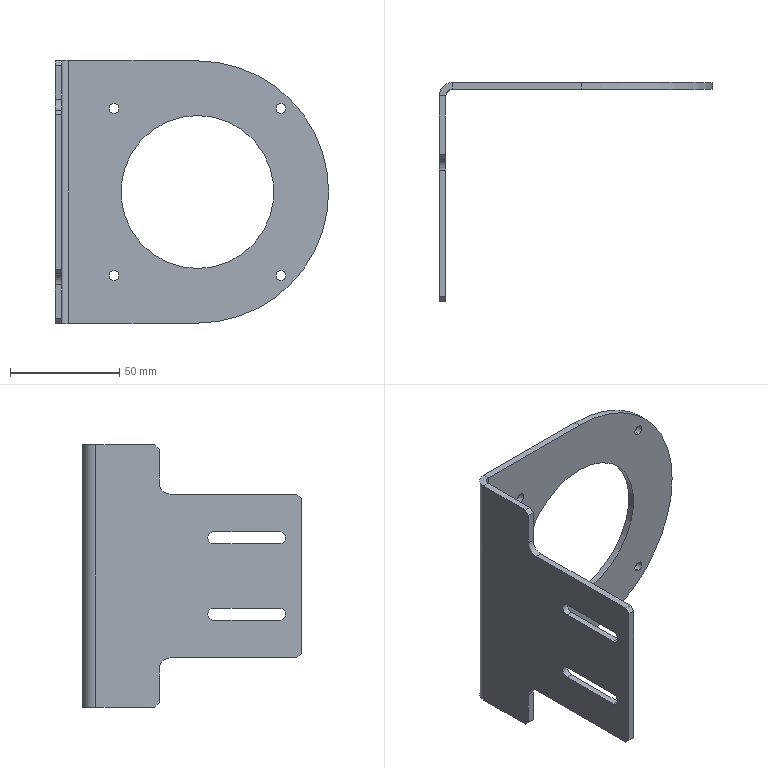Part | SolidWorks | features ICE 3, HoleWzd 2, Chamfer 1, EdgeFlange 1, Fillet 1, FlatPattern 1, MirrorSolid 1, SMBaseFlange 1, SheetMetal 1 | 1 solid | 42 faces | box 125 x 100 x 120 mm | volume 52954 mm3 | plane 23 | cylinder 19 | commonest cylinder face diameters 4.5 x8 5.5 x4 10 x2 70 x2 6 x1 12 x1
STEP:
#1=CARTESIAN_POINT('',(38.184,-3.,-40.434));
#2=VERTEX_POINT('',#1);
#3=CARTESIAN_POINT('',(38.184,-3.,-35.934));
#4=VERTEX_POINT('',#3);
#5=CARTESIAN_POINT('',(38.184,-3.,-38.184));
#6=DIRECTION('',(0.,1.,0.));
#7=DIRECTION('',(0.,0.,1.));
#8=AXIS2_PLACEMENT_3D('',#5,#6,#7);
#9=CIRCLE('',#8,2.25);
#10=EDGE_CURVE('',#2,#4,#9,.T.);
#11=ORIENTED_EDGE('',*,*,#10,.F.);
#12=CARTESIAN_POINT('',(38.184,0.,-40.434));
#13=VERTEX_POINT('',#12);
#14=CARTESIAN_POINT('',(38.184,0.,-40.434));
#15=DIRECTION('',(0.,1.,0.));
#16=VECTOR('',#15,1000.);
#17=LINE('',#14,#16);
#18=EDGE_CURVE('',#2,#13,#17,.T.);
#19=ORIENTED_EDGE('',*,*,#18,.T.);
#20=CARTESIAN_POINT('',(38.184,0.,-35.934));
#21=VERTEX_POINT('',#20);
#22=CARTESIAN_POINT('',(38.184,0.,-38.184));
#23=DIRECTION('',(0.,1.,0.));
#24=DIRECTION('',(0.,0.,1.));
#25=AXIS2_PLACEMENT_3D('',#22,#23,#24);
#26=CIRCLE('',#25,2.25);
#27=EDGE_CURVE('',#13,#21,#26,.T.);
#28=ORIENTED_EDGE('',*,*,#27,.T.);
#29=CARTESIAN_POINT('',(38.184,0.,-35.934));
#30=DIRECTION('',(0.,1.,0.));
#31=VECTOR('',#30,1000.);
#32=LINE('',#29,#31);
#33=EDGE_CURVE('',#4,#21,#32,.T.);
#34=ORIENTED_EDGE('',*,*,#33,.F.);
#35=EDGE_LOOP('',(#11,#19,#28,#34));
#36=FACE_OUTER_BOUND('',#35,.T.);
#37=CARTESIAN_POINT('',(38.184,0.,-38.184));
#38=DIRECTION('',(0.,1.,0.));
#39=DIRECTION('',(0.,0.,1.));
#40=AXIS2_PLACEMENT_3D('',#37,#38,#39);
#41=CYLINDRICAL_SURFACE('',#40,2.25);
#42=ADVANCED_FACE('',(#36),#41,.F.);
#43=CARTESIAN_POINT('',(38.184,-3.,35.934));
#44=VERTEX_POINT('',#43);
#45=CARTESIAN_POINT('',(38.184,-3.,40.434));
#46=VERTEX_POINT('',#45);
#47=CARTESIAN_POINT('',(38.184,-3.,38.184));
#48=DIRECTION('',(0.,1.,0.));
#49=DIRECTION('',(0.,0.,1.));
#50=AXIS2_PLACEMENT_3D('',#47,#48,#49);
#51=CIRCLE('',#50,2.25);
#52=EDGE_CURVE('',#44,#46,#51,.T.);
#53=ORIENTED_EDGE('',*,*,#52,.F.);
#54=CARTESIAN_POINT('',(38.184,0.,35.934));
#55=VERTEX_POINT('',#54);
#56=CARTESIAN_POINT('',(38.184,0.,35.934));
#57=DIRECTION('',(0.,1.,0.));
#58=VECTOR('',#57,1000.);
#59=LINE('',#56,#58);
#60=EDGE_CURVE('',#44,#55,#59,.T.);
#61=ORIENTED_EDGE('',*,*,#60,.T.);
#62=CARTESIAN_POINT('',(38.184,0.,40.434));
#63=VERTEX_POINT('',#62);
#64=CARTESIAN_POINT('',(38.184,0.,38.184));
#65=DIRECTION('',(0.,1.,0.));
#66=DIRECTION('',(0.,0.,1.));
#67=AXIS2_PLACEMENT_3D('',#64,#65,#66);
#68=CIRCLE('',#67,2.25);
#69=EDGE_CURVE('',#55,#63,#68,.T.);
#70=ORIENTED_EDGE('',*,*,#69,.T.);
#71=CARTESIAN_POINT('',(38.184,0.,40.434));
#72=DIRECTION('',(0.,1.,0.));
#73=VECTOR('',#72,1000.);
#74=LINE('',#71,#73);
#75=EDGE_CURVE('',#46,#63,#74,.T.);
#76=ORIENTED_EDGE('',*,*,#75,.F.);
#77=EDGE_LOOP('',(#53,#61,#70,#76));
#78=FACE_OUTER_BOUND('',#77,.T.);
#79=CARTESIAN_POINT('',(38.184,0.,38.184));
#80=DIRECTION('',(0.,1.,0.));
#81=DIRECTION('',(0.,0.,1.));
#82=AXIS2_PLACEMENT_3D('',#79,#80,#81);
#83=CYLINDRICAL_SURFACE('',#82,2.25);
#84=ADVANCED_FACE('',(#78),#83,.F.);
#85=CARTESIAN_POINT('',(-38.184,-3.,35.934));
#86=VERTEX_POINT('',#85);
#87=CARTESIAN_POINT('',(-38.184,-3.,40.434));
#88=VERTEX_POINT('',#87);
#89=CARTESIAN_POINT('',(-38.184,-3.,38.184));
#90=DIRECTION('',(0.,1.,0.));
#91=DIRECTION('',(0.,0.,1.));
#92=AXIS2_PLACEMENT_3D('',#89,#90,#91);
#93=CIRCLE('',#92,2.25);
#94=EDGE_CURVE('',#86,#88,#93,.T.);
#95=ORIENTED_EDGE('',*,*,#94,.F.);
#96=CARTESIAN_POINT('',(-38.184,0.,35.934));
#97=VERTEX_POINT('',#96);
#98=CARTESIAN_POINT('',(-38.184,0.,35.934));
#99=DIRECTION('',(0.,1.,0.));
#100=VECTOR('',#99,1000.);
#101=LINE('',#98,#100);
#102=EDGE_CURVE('',#86,#97,#101,.T.);
#103=ORIENTED_EDGE('',*,*,#102,.T.);
#104=CARTESIAN_POINT('',(-38.184,0.,40.434));
#105=VERTEX_POINT('',#104);
#106=CARTESIAN_POINT('',(-38.184,0.,38.184));
#107=DIRECTION('',(0.,1.,0.));
#108=DIRECTION('',(0.,0.,1.));
#109=AXIS2_PLACEMENT_3D('',#106,#107,#108);
#110=CIRCLE('',#109,2.25);
#111=EDGE_CURVE('',#97,#105,#110,.T.);
#112=ORIENTED_EDGE('',*,*,#111,.T.);
#113=CARTESIAN_POINT('',(-38.184,0.,40.434));
#114=DIRECTION('',(0.,1.,0.));
#115=VECTOR('',#114,1000.);
#116=LINE('',#113,#115);
#117=EDGE_CURVE('',#88,#105,#116,.T.);
#118=ORIENTED_EDGE('',*,*,#117,.F.);
#119=EDGE_LOOP('',(#95,#103,#112,#118));
#120=FACE_OUTER_BOUND('',#119,.T.);
#121=CARTESIAN_POINT('',(-38.184,0.,38.184));
#122=DIRECTION('',(0.,1.,0.));
#123=DIRECTION('',(0.,0.,1.));
#124=AXIS2_PLACEMENT_3D('',#121,#122,#123);
#125=CYLINDRICAL_SURFACE('',#124,2.25);
#126=ADVANCED_FACE('',(#120),#125,.F.);
#127=CARTESIAN_POINT('',(-38.184,-3.,-40.434));
#128=VERTEX_POINT('',#127);
#129=CARTESIAN_POINT('',(-38.184,-3.,-35.934));
#130=VERTEX_POINT('',#129);
#131=CARTESIAN_POINT('',(-38.184,-3.,-38.184));
#132=DIRECTION('',(0.,1.,0.));
#133=DIRECTION('',(0.,0.,1.));
#134=AXIS2_PLACEMENT_3D('',#131,#132,#133);
#135=CIRCLE('',#134,2.25);
#136=EDGE_CURVE('',#128,#130,#135,.T.);
#137=ORIENTED_EDGE('',*,*,#136,.F.);
#138=CARTESIAN_POINT('',(-38.184,0.,-40.434));
#139=VERTEX_POINT('',#138);
#140=CARTESIAN_POINT('',(-38.184,0.,-40.434));
#141=DIRECTION('',(0.,1.,0.));
#142=VECTOR('',#141,1000.);
#143=LINE('',#140,#142);
#144=EDGE_CURVE('',#128,#139,#143,.T.);
#145=ORIENTED_EDGE('',*,*,#144,.T.);
#146=CARTESIAN_POINT('',(-38.184,0.,-35.934));
#147=VERTEX_POINT('',#146);
#148=CARTESIAN_POINT('',(-38.184,0.,-38.184));
#149=DIRECTION('',(0.,1.,0.));
#150=DIRECTION('',(0.,0.,1.));
#151=AXIS2_PLACEMENT_3D('',#148,#149,#150);
#152=CIRCLE('',#151,2.25);
#153=EDGE_CURVE('',#139,#147,#152,.T.);
#154=ORIENTED_EDGE('',*,*,#153,.T.);
#155=CARTESIAN_POINT('',(-38.184,0.,-35.934));
#156=DIRECTION('',(0.,1.,0.));
#157=VECTOR('',#156,1000.);
#158=LINE('',#155,#157);
#159=EDGE_CURVE('',#130,#147,#158,.T.);
#160=ORIENTED_EDGE('',*,*,#159,.F.);
#161=EDGE_LOOP('',(#137,#145,#154,#160));
#162=FACE_OUTER_BOUND('',#161,.T.);
#163=CARTESIAN_POINT('',(-38.184,0.,-38.184));
#164=DIRECTION('',(0.,1.,0.));
#165=DIRECTION('',(0.,0.,1.));
#166=AXIS2_PLACEMENT_3D('',#163,#164,#165);
#167=CYLINDRICAL_SURFACE('',#166,2.25);
#168=ADVANCED_FACE('',(#162),#167,.F.);
#169=CARTESIAN_POINT('',(0.,-3.,-35.));
#170=VERTEX_POINT('',#169);
#171=CARTESIAN_POINT('',(0.,-3.,35.));
#172=VERTEX_POINT('',#171);
#173=CARTESIAN_POINT('',(0.,-3.,0.));
#174=DIRECTION('',(0.,1.,0.));
#175=DIRECTION('',(0.,0.,1.));
#176=AXIS2_PLACEMENT_3D('',#173,#174,#175);
#177=CIRCLE('',#176,35.);
#178=EDGE_CURVE('',#170,#172,#177,.T.);
#179=ORIENTED_EDGE('',*,*,#178,.F.);
#180=CARTESIAN_POINT('',(0.,0.,-35.));
#181=VERTEX_POINT('',#180);
#182=CARTESIAN_POINT('',(0.,-3.,-35.));
#183=DIRECTION('',(0.,1.,0.));
#184=VECTOR('',#183,1000.);
#185=LINE('',#182,#184);
#186=EDGE_CURVE('',#170,#181,#185,.T.);
#187=ORIENTED_EDGE('',*,*,#186,.T.);
#188=CARTESIAN_POINT('',(0.,0.,35.));
#189=VERTEX_POINT('',#188);
#190=CARTESIAN_POINT('',(0.,0.,0.));
#191=DIRECTION('',(0.,1.,0.));
#192=DIRECTION('',(0.,0.,1.));
#193=AXIS2_PLACEMENT_3D('',#190,#191,#192);
#194=CIRCLE('',#193,35.);
#195=EDGE_CURVE('',#181,#189,#194,.T.);
#196=ORIENTED_EDGE('',*,*,#195,.T.);
#197=CARTESIAN_POINT('',(0.,-3.,35.));
#198=DIRECTION('',(0.,1.,0.));
#199=VECTOR('',#198,1000.);
#200=LINE('',#197,#199);
#201=EDGE_CURVE('',#172,#189,#200,.T.);
#202=ORIENTED_EDGE('',*,*,#201,.F.);
#203=EDGE_LOOP('',(#179,#187,#196,#202));
#204=FACE_OUTER_BOUND('',#203,.T.);
#205=CARTESIAN_POINT('',(0.,-3.,0.));
#206=DIRECTION('',(0.,1.,0.));
#207=DIRECTION('',(0.,0.,1.));
#208=AXIS2_PLACEMENT_3D('',#205,#206,#207);
#209=CYLINDRICAL_SURFACE('',#208,35.);
#210=ADVANCED_FACE('',(#204),#209,.F.);
#211=CARTESIAN_POINT('',(0.,-3.,-60.));
#212=VERTEX_POINT('',#211);
#213=CARTESIAN_POINT('',(-59.,-3.,-60.));
#214=VERTEX_POINT('',#213);
#215=CARTESIAN_POINT('',(0.,-3.,-60.));
#216=DIRECTION('',(-1.,0.,0.));
#217=VECTOR('',#216,1000.);
#218=LINE('',#215,#217);
#219=EDGE_CURVE('',#212,#214,#218,.T.);
#220=ORIENTED_EDGE('',*,*,#219,.T.);
#221=CARTESIAN_POINT('',(-59.,0.,-60.));
#222=VERTEX_POINT('',#221);
#223=CARTESIAN_POINT('',(-59.,-3.,-60.));
#224=DIRECTION('',(0.,1.,0.));
#225=VECTOR('',#224,1000.);
#226=LINE('',#223,#225);
#227=EDGE_CURVE('',#214,#222,#226,.T.);
#228=ORIENTED_EDGE('',*,*,#227,.T.);
#229=CARTESIAN_POINT('',(0.,0.,-60.));
#230=VERTEX_POINT('',#229);
#231=CARTESIAN_POINT('',(0.,0.,-60.));
#232=DIRECTION('',(-1.,0.,0.));
#233=VECTOR('',#232,1000.);
#234=LINE('',#231,#233);
#235=EDGE_CURVE('',#230,#222,#234,.T.);
#236=ORIENTED_EDGE('',*,*,#235,.F.);
#237=CARTESIAN_POINT('',(0.,-3.,-60.));
#238=DIRECTION('',(0.,1.,0.));
#239=VECTOR('',#238,1000.);
#240=LINE('',#237,#239);
#241=EDGE_CURVE('',#212,#230,#240,.T.);
#242=ORIENTED_EDGE('',*,*,#241,.F.);
#243=EDGE_LOOP('',(#220,#228,#236,#242));
#244=FACE_OUTER_BOUND('',#243,.T.);
#245=CARTESIAN_POINT('',(0.,-3.,-60.));
#246=DIRECTION('',(0.,0.,-1.));
#247=DIRECTION('',(-1.,0.,0.));
#248=AXIS2_PLACEMENT_3D('',#245,#246,#247);
#249=PLANE('',#248);
#250=ADVANCED_FACE('',(#244),#249,.T.);
#251=CARTESIAN_POINT('',(38.184,-3.,-38.184));
#252=DIRECTION('',(0.,1.,0.));
#253=DIRECTION('',(0.,0.,1.));
#254=AXIS2_PLACEMENT_3D('',#251,#252,#253);
#255=CIRCLE('',#254,2.25);
#256=EDGE_CURVE('',#4,#2,#255,.T.);
#257=ORIENTED_EDGE('',*,*,#256,.T.);
#258=ORIENTED_EDGE('',*,*,#10,.T.);
#259=EDGE_LOOP('',(#257,#258));
#260=FACE_BOUND('',#259,.T.);
#261=CARTESIAN_POINT('',(38.184,-3.,38.184));
#262=DIRECTION('',(0.,1.,0.));
#263=DIRECTION('',(0.,0.,1.));
#264=AXIS2_PLACEMENT_3D('',#261,#262,#263);
#265=CIRCLE('',#264,2.25);
#266=EDGE_CURVE('',#46,#44,#265,.T.);
#267=ORIENTED_EDGE('',*,*,#266,.T.);
#268=ORIENTED_EDGE('',*,*,#52,.T.);
#269=EDGE_LOOP('',(#267,#268));
#270=FACE_BOUND('',#269,.T.);
#271=CARTESIAN_POINT('',(-38.184,-3.,38.184));
#272=DIRECTION('',(0.,1.,0.));
#273=DIRECTION('',(0.,0.,1.));
#274=AXIS2_PLACEMENT_3D('',#271,#272,#273);
#275=CIRCLE('',#274,2.25);
#276=EDGE_CURVE('',#88,#86,#275,.T.);
#277=ORIENTED_EDGE('',*,*,#276,.T.);
#278=ORIENTED_EDGE('',*,*,#94,.T.);
#279=EDGE_LOOP('',(#277,#278));
#280=FACE_BOUND('',#279,.T.);
#281=CARTESIAN_POINT('',(-38.184,-3.,-38.184));
#282=DIRECTION('',(0.,1.,0.));
#283=DIRECTION('',(0.,0.,1.));
#284=AXIS2_PLACEMENT_3D('',#281,#282,#283);
#285=CIRCLE('',#284,2.25);
#286=EDGE_CURVE('',#130,#128,#285,.T.);
#287=ORIENTED_EDGE('',*,*,#286,.T.);
#288=ORIENTED_EDGE('',*,*,#136,.T.);
#289=EDGE_LOOP('',(#287,#288));
#290=FACE_BOUND('',#289,.T.);
#291=CARTESIAN_POINT('',(0.,-3.,0.));
#292=DIRECTION('',(0.,1.,0.));
#293=DIRECTION('',(0.,0.,1.));
#294=AXIS2_PLACEMENT_3D('',#291,#292,#293);
#295=CIRCLE('',#294,35.);
#296=EDGE_CURVE('',#172,#170,#295,.T.);
#297=ORIENTED_EDGE('',*,*,#296,.T.);
#298=ORIENTED_EDGE('',*,*,#178,.T.);
#299=EDGE_LOOP('',(#297,#298));
#300=FACE_BOUND('',#299,.T.);
#301=CARTESIAN_POINT('',(-59.,-3.,60.));
#302=VERTEX_POINT('',#301);
#303=CARTESIAN_POINT('',(-59.,-3.,-60.));
#304=DIRECTION('',(0.,0.,1.));
#305=VECTOR('',#304,1000.);
#306=LINE('',#303,#305);
#307=EDGE_CURVE('',#214,#302,#306,.T.);
#308=ORIENTED_EDGE('',*,*,#307,.F.);
#309=ORIENTED_EDGE('',*,*,#219,.F.);
#310=CARTESIAN_POINT('',(0.,-3.,60.));
#311=VERTEX_POINT('',#310);
#312=CARTESIAN_POINT('',(0.,-3.,0.));
#313=DIRECTION('',(0.,1.,0.));
#314=DIRECTION('',(0.,0.,1.));
#315=AXIS2_PLACEMENT_3D('',#312,#313,#314);
#316=CIRCLE('',#315,60.);
#317=EDGE_CURVE('',#311,#212,#316,.T.);
#318=ORIENTED_EDGE('',*,*,#317,.F.);
#319=CARTESIAN_POINT('',(-65.,-3.,60.));
#320=DIRECTION('',(1.,0.,0.));
#321=VECTOR('',#320,1000.);
#322=LINE('',#319,#321);
#323=EDGE_CURVE('',#302,#311,#322,.T.);
#324=ORIENTED_EDGE('',*,*,#323,.F.);
#325=EDGE_LOOP('',(#308,#309,#318,#324));
#326=FACE_OUTER_BOUND('',#325,.T.);
#327=CARTESIAN_POINT('',(0.,-3.,0.));
#328=DIRECTION('',(0.,1.,0.));
#329=DIRECTION('',(0.,0.,1.));
#330=AXIS2_PLACEMENT_3D('',#327,#328,#329);
#331=PLANE('',#330);
#332=ADVANCED_FACE('',(#260,#270,#280,#290,#300,#326),#331,.F.);
#333=CARTESIAN_POINT('',(38.184,0.,-38.184));
#334=DIRECTION('',(0.,1.,0.));
#335=DIRECTION('',(0.,0.,1.));
#336=AXIS2_PLACEMENT_3D('',#333,#334,#335);
#337=CIRCLE('',#336,2.25);
#338=EDGE_CURVE('',#21,#13,#337,.T.);
#339=ORIENTED_EDGE('',*,*,#338,.F.);
#340=ORIENTED_EDGE('',*,*,#27,.F.);
#341=EDGE_LOOP('',(#339,#340));
#342=FACE_BOUND('',#341,.T.);
#343=CARTESIAN_POINT('',(38.184,0.,38.184));
#344=DIRECTION('',(0.,1.,0.));
#345=DIRECTION('',(0.,0.,1.));
#346=AXIS2_PLACEMENT_3D('',#343,#344,#345);
#347=CIRCLE('',#346,2.25);
#348=EDGE_CURVE('',#63,#55,#347,.T.);
#349=ORIENTED_EDGE('',*,*,#348,.F.);
#350=ORIENTED_EDGE('',*,*,#69,.F.);
#351=EDGE_LOOP('',(#349,#350));
#352=FACE_BOUND('',#351,.T.);
#353=CARTESIAN_POINT('',(-38.184,0.,38.184));
#354=DIRECTION('',(0.,1.,0.));
#355=DIRECTION('',(0.,0.,1.));
#356=AXIS2_PLACEMENT_3D('',#353,#354,#355);
#357=CIRCLE('',#356,2.25);
#358=EDGE_CURVE('',#105,#97,#357,.T.);
#359=ORIENTED_EDGE('',*,*,#358,.F.);
#360=ORIENTED_EDGE('',*,*,#111,.F.);
#361=EDGE_LOOP('',(#359,#360));
#362=FACE_BOUND('',#361,.T.);
#363=CARTESIAN_POINT('',(-38.184,0.,-38.184));
#364=DIRECTION('',(0.,1.,0.));
#365=DIRECTION('',(0.,0.,1.));
#366=AXIS2_PLACEMENT_3D('',#363,#364,#365);
#367=CIRCLE('',#366,2.25);
#368=EDGE_CURVE('',#147,#139,#367,.T.);
#369=ORIENTED_EDGE('',*,*,#368,.F.);
#370=ORIENTED_EDGE('',*,*,#153,.F.);
#371=EDGE_LOOP('',(#369,#370));
#372=FACE_BOUND('',#371,.T.);
#373=CARTESIAN_POINT('',(0.,0.,0.));
#374=DIRECTION('',(0.,1.,0.));
#375=DIRECTION('',(0.,0.,1.));
#376=AXIS2_PLACEMENT_3D('',#373,#374,#375);
#377=CIRCLE('',#376,35.);
#378=EDGE_CURVE('',#189,#181,#377,.T.);
#379=ORIENTED_EDGE('',*,*,#378,.F.);
#380=ORIENTED_EDGE('',*,*,#195,.F.);
#381=EDGE_LOOP('',(#379,#380));
#382=FACE_BOUND('',#381,.T.);
#383=ORIENTED_EDGE('',*,*,#235,.T.);
#384=CARTESIAN_POINT('',(-59.,0.,60.));
#385=VERTEX_POINT('',#384);
#386=CARTESIAN_POINT('',(-59.,0.,-60.));
#387=DIRECTION('',(0.,0.,1.));
#388=VECTOR('',#387,1000.);
#389=LINE('',#386,#388);
#390=EDGE_CURVE('',#222,#385,#389,.T.);
#391=ORIENTED_EDGE('',*,*,#390,.T.);
#392=CARTESIAN_POINT('',(0.,0.,60.));
#393=VERTEX_POINT('',#392);
#394=CARTESIAN_POINT('',(-65.,0.,60.));
#395=DIRECTION('',(1.,0.,0.));
#396=VECTOR('',#395,1000.);
#397=LINE('',#394,#396);
#398=EDGE_CURVE('',#385,#393,#397,.T.);
#399=ORIENTED_EDGE('',*,*,#398,.T.);
#400=CARTESIAN_POINT('',(0.,0.,0.));
#401=DIRECTION('',(0.,1.,0.));
#402=DIRECTION('',(0.,0.,1.));
#403=AXIS2_PLACEMENT_3D('',#400,#401,#402);
#404=CIRCLE('',#403,60.);
#405=EDGE_CURVE('',#393,#230,#404,.T.);
#406=ORIENTED_EDGE('',*,*,#405,.T.);
#407=EDGE_LOOP('',(#383,#391,#399,#406));
#408=FACE_OUTER_BOUND('',#407,.T.);
#409=CARTESIAN_POINT('',(0.,0.,0.));
#410=DIRECTION('',(0.,1.,0.));
#411=DIRECTION('',(0.,0.,1.));
#412=AXIS2_PLACEMENT_3D('',#409,#410,#411);
#413=PLANE('',#412);
#414=ADVANCED_FACE('',(#342,#352,#362,#372,#382,#408),#413,.T.);
#415=ORIENTED_EDGE('',*,*,#405,.F.);
#416=CARTESIAN_POINT('',(0.,-3.,60.));
#417=DIRECTION('',(0.,1.,0.));
#418=VECTOR('',#417,1000.);
#419=LINE('',#416,#418);
#420=EDGE_CURVE('',#311,#393,#419,.T.);
#421=ORIENTED_EDGE('',*,*,#420,.F.);
#422=ORIENTED_EDGE('',*,*,#317,.T.);
#423=ORIENTED_EDGE('',*,*,#241,.T.);
#424=EDGE_LOOP('',(#415,#421,#422,#423));
#425=FACE_OUTER_BOUND('',#424,.T.);
#426=CARTESIAN_POINT('',(0.,-3.,0.));
#427=DIRECTION('',(0.,1.,0.));
#428=DIRECTION('',(0.,0.,1.));
#429=AXIS2_PLACEMENT_3D('',#426,#427,#428);
#430=CYLINDRICAL_SURFACE('',#429,60.);
#431=ADVANCED_FACE('',(#425),#430,.T.);
#432=CARTESIAN_POINT('',(-59.,-3.,60.));
#433=DIRECTION('',(0.,1.,0.));
#434=VECTOR('',#433,1000.);
#435=LINE('',#432,#434);
#436=EDGE_CURVE('',#302,#385,#435,.T.);
#437=ORIENTED_EDGE('',*,*,#436,.F.);
#438=ORIENTED_EDGE('',*,*,#323,.T.);
#439=ORIENTED_EDGE('',*,*,#420,.T.);
#440=ORIENTED_EDGE('',*,*,#398,.F.);
#441=EDGE_LOOP('',(#437,#438,#439,#440));
#442=FACE_OUTER_BOUND('',#441,.T.);
#443=CARTESIAN_POINT('',(-65.,-3.,60.));
#444=DIRECTION('',(0.,0.,1.));
#445=DIRECTION('',(1.,0.,0.));
#446=AXIS2_PLACEMENT_3D('',#443,#444,#445);
#447=PLANE('',#446);
#448=ADVANCED_FACE('',(#442),#447,.T.);
#449=ORIENTED_EDGE('',*,*,#186,.F.);
#450=ORIENTED_EDGE('',*,*,#296,.F.);
#451=ORIENTED_EDGE('',*,*,#201,.T.);
#452=ORIENTED_EDGE('',*,*,#378,.T.);
#453=EDGE_LOOP('',(#449,#450,#451,#452));
#454=FACE_OUTER_BOUND('',#453,.T.);
#455=CARTESIAN_POINT('',(0.,-3.,0.));
#456=DIRECTION('',(0.,1.,0.));
#457=DIRECTION('',(0.,0.,1.));
#458=AXIS2_PLACEMENT_3D('',#455,#456,#457);
#459=CYLINDRICAL_SURFACE('',#458,35.);
#460=ADVANCED_FACE('',(#454),#459,.F.);
#461=CARTESIAN_POINT('',(-62.,-6.,60.));
#462=VERTEX_POINT('',#461);
#463=CARTESIAN_POINT('',(-65.,-6.,60.));
#464=VERTEX_POINT('',#463);
#465=CARTESIAN_POINT('',(-65.,-6.,60.));
#466=DIRECTION('',(-1.,0.,0.));
#467=VECTOR('',#466,1000.);
#468=LINE('',#465,#467);
#469=EDGE_CURVE('',#462,#464,#468,.T.);
#470=ORIENTED_EDGE('',*,*,#469,.F.);
#471=CARTESIAN_POINT('',(-59.,-6.,60.));
#472=DIRECTION('',(0.,0.,1.));
#473=DIRECTION('',(-1.,0.,0.));
#474=AXIS2_PLACEMENT_3D('',#471,#472,#473);
#475=CIRCLE('',#474,3.);
#476=EDGE_CURVE('',#302,#462,#475,.T.);
#477=ORIENTED_EDGE('',*,*,#476,.F.);
#478=ORIENTED_EDGE('',*,*,#436,.T.);
#479=CARTESIAN_POINT('',(-59.,-6.,60.));
#480=DIRECTION('',(0.,0.,1.));
#481=DIRECTION('',(-1.,0.,0.));
#482=AXIS2_PLACEMENT_3D('',#479,#480,#481);
#483=CIRCLE('',#482,6.);
#484=EDGE_CURVE('',#385,#464,#483,.T.);
#485=ORIENTED_EDGE('',*,*,#484,.T.);
#486=EDGE_LOOP('',(#470,#477,#478,#485));
#487=FACE_OUTER_BOUND('',#486,.T.);
#488=CARTESIAN_POINT('',(-59.,-6.,60.));
#489=DIRECTION('',(0.,0.,1.));
#490=DIRECTION('',(1.,0.,0.));
#491=AXIS2_PLACEMENT_3D('',#488,#489,#490);
#492=PLANE('',#491);
#493=ADVANCED_FACE('',(#487),#492,.T.);
#494=CARTESIAN_POINT('',(-62.,-6.,-60.));
#495=VERTEX_POINT('',#494);
#496=CARTESIAN_POINT('',(-59.,-6.,-60.));
#497=DIRECTION('',(0.,0.,-1.));
#498=DIRECTION('',(-1.,0.,0.));
#499=AXIS2_PLACEMENT_3D('',#496,#497,#498);
#500=CIRCLE('',#499,3.);
#501=EDGE_CURVE('',#495,#214,#500,.T.);
#502=ORIENTED_EDGE('',*,*,#501,.F.);
#503=CARTESIAN_POINT('',(-65.,-6.,-60.));
#504=VERTEX_POINT('',#503);
#505=CARTESIAN_POINT('',(-62.,-6.,-60.));
#506=DIRECTION('',(-1.,0.,0.));
#507=VECTOR('',#506,1000.);
#508=LINE('',#505,#507);
#509=EDGE_CURVE('',#495,#504,#508,.T.);
#510=ORIENTED_EDGE('',*,*,#509,.T.);
#511=CARTESIAN_POINT('',(-59.,-6.,-60.));
#512=DIRECTION('',(0.,0.,-1.));
#513=DIRECTION('',(-1.,0.,0.));
#514=AXIS2_PLACEMENT_3D('',#511,#512,#513);
#515=CIRCLE('',#514,6.);
#516=EDGE_CURVE('',#504,#222,#515,.T.);
#517=ORIENTED_EDGE('',*,*,#516,.T.);
#518=ORIENTED_EDGE('',*,*,#227,.F.);
#519=EDGE_LOOP('',(#502,#510,#517,#518));
#520=FACE_OUTER_BOUND('',#519,.T.);
#521=CARTESIAN_POINT('',(-59.,-6.,-60.));
#522=DIRECTION('',(0.,0.,1.));
#523=DIRECTION('',(1.,0.,0.));
#524=AXIS2_PLACEMENT_3D('',#521,#522,#523);
#525=PLANE('',#524);
#526=ADVANCED_FACE('',(#520),#525,.F.);
#527=ORIENTED_EDGE('',*,*,#390,.F.);
#528=ORIENTED_EDGE('',*,*,#516,.F.);
#529=CARTESIAN_POINT('',(-65.,-6.,0.));
#530=DIRECTION('',(0.,0.,-1.));
#531=VECTOR('',#530,1000.);
#532=LINE('',#529,#531);
#533=EDGE_CURVE('',#464,#504,#532,.T.);
#534=ORIENTED_EDGE('',*,*,#533,.F.);
#535=ORIENTED_EDGE('',*,*,#484,.F.);
#536=EDGE_LOOP('',(#527,#528,#534,#535));
#537=FACE_OUTER_BOUND('',#536,.T.);
#538=CARTESIAN_POINT('',(-59.,-6.,-60.));
#539=DIRECTION('',(0.,0.,-1.));
#540=DIRECTION('',(-1.,0.,0.));
#541=AXIS2_PLACEMENT_3D('',#538,#539,#540);
#542=CYLINDRICAL_SURFACE('',#541,6.);
#543=ADVANCED_FACE('',(#537),#542,.T.);
#544=ORIENTED_EDGE('',*,*,#307,.T.);
#545=ORIENTED_EDGE('',*,*,#476,.T.);
#546=CARTESIAN_POINT('',(-62.,-6.,60.));
#547=DIRECTION('',(0.,0.,-1.));
#548=VECTOR('',#547,1000.);
#549=LINE('',#546,#548);
#550=EDGE_CURVE('',#462,#495,#549,.T.);
#551=ORIENTED_EDGE('',*,*,#550,.T.);
#552=ORIENTED_EDGE('',*,*,#501,.T.);
#553=EDGE_LOOP('',(#544,#545,#551,#552));
#554=FACE_OUTER_BOUND('',#553,.T.);
#555=CARTESIAN_POINT('',(-59.,-6.,-60.));
#556=DIRECTION('',(0.,0.,-1.));
#557=DIRECTION('',(-1.,0.,0.));
#558=AXIS2_PLACEMENT_3D('',#555,#556,#557);
#559=CYLINDRICAL_SURFACE('',#558,3.);
#560=ADVANCED_FACE('',(#554),#559,.F.);
#561=CARTESIAN_POINT('',(-62.,-33.,-60.));
#562=VERTEX_POINT('',#561);
#563=CARTESIAN_POINT('',(-62.,0.,-60.));
#564=DIRECTION('',(0.,1.,0.));
#565=VECTOR('',#564,1000.);
#566=LINE('',#563,#565);
#567=EDGE_CURVE('',#562,#495,#566,.T.);
#568=ORIENTED_EDGE('',*,*,#567,.F.);
#569=CARTESIAN_POINT('',(-65.,-33.,-60.));
#570=VERTEX_POINT('',#569);
#571=CARTESIAN_POINT('',(-65.,-33.,-60.));
#572=DIRECTION('',(-1.,0.,0.));
#573=VECTOR('',#572,1000.);
#574=LINE('',#571,#573);
#575=EDGE_CURVE('',#562,#570,#574,.T.);
#576=ORIENTED_EDGE('',*,*,#575,.T.);
#577=CARTESIAN_POINT('',(-65.,-3.,-60.));
#578=DIRECTION('',(0.,1.,0.));
#579=VECTOR('',#578,1000.);
#580=LINE('',#577,#579);
#581=EDGE_CURVE('',#570,#504,#580,.T.);
#582=ORIENTED_EDGE('',*,*,#581,.T.);
#583=ORIENTED_EDGE('',*,*,#509,.F.);
#584=EDGE_LOOP('',(#568,#576,#582,#583));
#585=FACE_OUTER_BOUND('',#584,.T.);
#586=CARTESIAN_POINT('',(-65.,-3.,-60.));
#587=DIRECTION('',(0.,0.,-1.));
#588=DIRECTION('',(-1.,0.,0.));
#589=AXIS2_PLACEMENT_3D('',#586,#587,#588);
#590=PLANE('',#589);
#591=ADVANCED_FACE('',(#585),#590,.T.);
#592=CARTESIAN_POINT('',(-65.,-33.,60.));
#593=VERTEX_POINT('',#592);
#594=CARTESIAN_POINT('',(-65.,-100.,60.));
#595=DIRECTION('',(0.,-1.,0.));
#596=VECTOR('',#595,1000.);
#597=LINE('',#594,#596);
#598=EDGE_CURVE('',#464,#593,#597,.T.);
#599=ORIENTED_EDGE('',*,*,#598,.T.);
#600=CARTESIAN_POINT('',(-62.,-33.,60.));
#601=VERTEX_POINT('',#600);
#602=CARTESIAN_POINT('',(-62.,-33.,60.));
#603=DIRECTION('',(1.,0.,0.));
#604=VECTOR('',#603,1000.);
#605=LINE('',#602,#604);
#606=EDGE_CURVE('',#593,#601,#605,.T.);
#607=ORIENTED_EDGE('',*,*,#606,.T.);
#608=CARTESIAN_POINT('',(-62.,0.,60.));
#609=DIRECTION('',(0.,-1.,0.));
#610=VECTOR('',#609,1000.);
#611=LINE('',#608,#610);
#612=EDGE_CURVE('',#462,#601,#611,.T.);
#613=ORIENTED_EDGE('',*,*,#612,.F.);
#614=ORIENTED_EDGE('',*,*,#469,.T.);
#615=EDGE_LOOP('',(#599,#607,#613,#614));
#616=FACE_OUTER_BOUND('',#615,.T.);
#617=CARTESIAN_POINT('',(-65.,-100.,60.));
#618=DIRECTION('',(0.,0.,1.));
#619=DIRECTION('',(0.,-1.,0.));
#620=AXIS2_PLACEMENT_3D('',#617,#618,#619);
#621=PLANE('',#620);
#622=ADVANCED_FACE('',(#616),#621,.T.);
#623=CARTESIAN_POINT('',(-65.,-90.,-14.75));
#624=VERTEX_POINT('',#623);
#625=CARTESIAN_POINT('',(-65.,-60.,-14.75));
#626=VERTEX_POINT('',#625);
#627=CARTESIAN_POINT('',(-65.,-90.,-14.75));
#628=DIRECTION('',(0.,1.,0.));
#629=VECTOR('',#628,1000.);
#630=LINE('',#627,#629);
#631=EDGE_CURVE('',#624,#626,#630,.T.);
#632=ORIENTED_EDGE('',*,*,#631,.F.);
#633=CARTESIAN_POINT('',(-65.,-90.,-20.25));
#634=VERTEX_POINT('',#633);
#635=CARTESIAN_POINT('',(-65.,-90.,-17.5));
#636=DIRECTION('',(-1.,0.,0.));
#637=DIRECTION('',(0.,0.,1.));
#638=AXIS2_PLACEMENT_3D('',#635,#636,#637);
#639=CIRCLE('',#638,2.75);
#640=EDGE_CURVE('',#634,#624,#639,.T.);
#641=ORIENTED_EDGE('',*,*,#640,.F.);
#642=CARTESIAN_POINT('',(-65.,-60.,-20.25));
#643=VERTEX_POINT('',#642);
#644=CARTESIAN_POINT('',(-65.,-90.,-20.25));
#645=DIRECTION('',(0.,1.,0.));
#646=VECTOR('',#645,1000.);
#647=LINE('',#644,#646);
#648=EDGE_CURVE('',#634,#643,#647,.T.);
#649=ORIENTED_EDGE('',*,*,#648,.T.);
#650=CARTESIAN_POINT('',(-65.,-60.,-17.5));
#651=DIRECTION('',(-1.,0.,0.));
#652=DIRECTION('',(0.,0.,1.));
#653=AXIS2_PLACEMENT_3D('',#650,#651,#652);
#654=CIRCLE('',#653,2.75);
#655=EDGE_CURVE('',#626,#643,#654,.T.);
#656=ORIENTED_EDGE('',*,*,#655,.F.);
#657=EDGE_LOOP('',(#632,#641,#649,#656));
#658=FACE_BOUND('',#657,.T.);
#659=CARTESIAN_POINT('',(-65.,-90.,20.25));
#660=VERTEX_POINT('',#659);
#661=CARTESIAN_POINT('',(-65.,-60.,20.25));
#662=VERTEX_POINT('',#661);
#663=CARTESIAN_POINT('',(-65.,-90.,20.25));
#664=DIRECTION('',(0.,1.,0.));
#665=VECTOR('',#664,1000.);
#666=LINE('',#663,#665);
#667=EDGE_CURVE('',#660,#662,#666,.T.);
#668=ORIENTED_EDGE('',*,*,#667,.F.);
#669=CARTESIAN_POINT('',(-65.,-90.,14.75));
#670=VERTEX_POINT('',#669);
#671=CARTESIAN_POINT('',(-65.,-90.,17.5));
#672=DIRECTION('',(-1.,0.,0.));
#673=DIRECTION('',(0.,0.,1.));
#674=AXIS2_PLACEMENT_3D('',#671,#672,#673);
#675=CIRCLE('',#674,2.75);
#676=EDGE_CURVE('',#670,#660,#675,.T.);
#677=ORIENTED_EDGE('',*,*,#676,.F.);
#678=CARTESIAN_POINT('',(-65.,-60.,14.75));
#679=VERTEX_POINT('',#678);
#680=CARTESIAN_POINT('',(-65.,-90.,14.75));
#681=DIRECTION('',(0.,1.,0.));
#682=VECTOR('',#681,1000.);
#683=LINE('',#680,#682);
#684=EDGE_CURVE('',#670,#679,#683,.T.);
#685=ORIENTED_EDGE('',*,*,#684,.T.);
#686=CARTESIAN_POINT('',(-65.,-60.,17.5));
#687=DIRECTION('',(-1.,0.,0.));
#688=DIRECTION('',(0.,0.,1.));
#689=AXIS2_PLACEMENT_3D('',#686,#687,#688);
#690=CIRCLE('',#689,2.75);
#691=EDGE_CURVE('',#662,#679,#690,.T.);
#692=ORIENTED_EDGE('',*,*,#691,.F.);
#693=EDGE_LOOP('',(#668,#677,#685,#692));
#694=FACE_BOUND('',#693,.T.);
#695=ORIENTED_EDGE('',*,*,#581,.F.);
#696=CARTESIAN_POINT('',(-65.,-35.,-58.));
#697=VERTEX_POINT('',#696);
#698=CARTESIAN_POINT('',(-65.,-46.5,-46.5));
#699=DIRECTION('',(0.,-0.7071,0.7071));
#700=VECTOR('',#699,1000.);
#701=LINE('',#698,#700);
#702=EDGE_CURVE('',#570,#697,#701,.T.);
#703=ORIENTED_EDGE('',*,*,#702,.T.);
#704=CARTESIAN_POINT('',(-65.,-35.,-42.5));
#705=VERTEX_POINT('',#704);
#706=CARTESIAN_POINT('',(-65.,-35.,-60.));
#707=DIRECTION('',(0.,0.,-1.));
#708=VECTOR('',#707,1000.);
#709=LINE('',#706,#708);
#710=EDGE_CURVE('',#705,#697,#709,.T.);
#711=ORIENTED_EDGE('',*,*,#710,.F.);
#712=CARTESIAN_POINT('',(-65.,-40.,-37.5));
#713=VERTEX_POINT('',#712);
#714=CARTESIAN_POINT('',(-65.,-40.,-42.5));
#715=DIRECTION('',(-1.,0.,0.));
#716=DIRECTION('',(0.,1.,0.));
#717=AXIS2_PLACEMENT_3D('',#714,#715,#716);
#718=CIRCLE('',#717,5.);
#719=EDGE_CURVE('',#713,#705,#718,.T.);
#720=ORIENTED_EDGE('',*,*,#719,.F.);
#721=CARTESIAN_POINT('',(-65.,-98.,-37.5));
#722=VERTEX_POINT('',#721);
#723=CARTESIAN_POINT('',(-65.,-100.,-37.5));
#724=DIRECTION('',(0.,1.,0.));
#725=VECTOR('',#724,1000.);
#726=LINE('',#723,#725);
#727=EDGE_CURVE('',#722,#713,#726,.T.);
#728=ORIENTED_EDGE('',*,*,#727,.F.);
#729=CARTESIAN_POINT('',(-65.,-100.,-35.5));
#730=VERTEX_POINT('',#729);
#731=CARTESIAN_POINT('',(-65.,-67.75,-67.75));
#732=DIRECTION('',(0.,-0.7071,0.7071));
#733=VECTOR('',#732,1000.);
#734=LINE('',#731,#733);
#735=EDGE_CURVE('',#722,#730,#734,.T.);
#736=ORIENTED_EDGE('',*,*,#735,.T.);
#737=CARTESIAN_POINT('',(-65.,-100.,35.5));
#738=VERTEX_POINT('',#737);
#739=CARTESIAN_POINT('',(-65.,-100.,-60.));
#740=DIRECTION('',(0.,0.,-1.));
#741=VECTOR('',#740,1000.);
#742=LINE('',#739,#741);
#743=EDGE_CURVE('',#738,#730,#742,.T.);
#744=ORIENTED_EDGE('',*,*,#743,.F.);
#745=CARTESIAN_POINT('',(-65.,-98.,37.5));
#746=VERTEX_POINT('',#745);
#747=CARTESIAN_POINT('',(-65.,-67.75,67.75));
#748=DIRECTION('',(0.,0.7071,0.7071));
#749=VECTOR('',#748,1000.);
#750=LINE('',#747,#749);
#751=EDGE_CURVE('',#738,#746,#750,.T.);
#752=ORIENTED_EDGE('',*,*,#751,.T.);
#753=CARTESIAN_POINT('',(-65.,-40.,37.5));
#754=VERTEX_POINT('',#753);
#755=CARTESIAN_POINT('',(-65.,-100.,37.5));
#756=DIRECTION('',(0.,-1.,0.));
#757=VECTOR('',#756,1000.);
#758=LINE('',#755,#757);
#759=EDGE_CURVE('',#754,#746,#758,.T.);
#760=ORIENTED_EDGE('',*,*,#759,.F.);
#761=CARTESIAN_POINT('',(-65.,-35.,42.5));
#762=VERTEX_POINT('',#761);
#763=CARTESIAN_POINT('',(-65.,-40.,42.5));
#764=DIRECTION('',(-1.,0.,0.));
#765=DIRECTION('',(0.,1.,0.));
#766=AXIS2_PLACEMENT_3D('',#763,#764,#765);
#767=CIRCLE('',#766,5.);
#768=EDGE_CURVE('',#762,#754,#767,.T.);
#769=ORIENTED_EDGE('',*,*,#768,.F.);
#770=CARTESIAN_POINT('',(-65.,-35.,58.));
#771=VERTEX_POINT('',#770);
#772=CARTESIAN_POINT('',(-65.,-35.,60.));
#773=DIRECTION('',(0.,0.,-1.));
#774=VECTOR('',#773,1000.);
#775=LINE('',#772,#774);
#776=EDGE_CURVE('',#771,#762,#775,.T.);
#777=ORIENTED_EDGE('',*,*,#776,.F.);
#778=CARTESIAN_POINT('',(-65.,-46.5,46.5));
#779=DIRECTION('',(0.,0.7071,0.7071));
#780=VECTOR('',#779,1000.);
#781=LINE('',#778,#780);
#782=EDGE_CURVE('',#771,#593,#781,.T.);
#783=ORIENTED_EDGE('',*,*,#782,.T.);
#784=ORIENTED_EDGE('',*,*,#598,.F.);
#785=ORIENTED_EDGE('',*,*,#533,.T.);
#786=EDGE_LOOP('',(#695,#703,#711,#720,#728,#736,#744,#752,#760,#769,#777,#783,#784,#785));
#787=FACE_OUTER_BOUND('',#786,.T.);
#788=CARTESIAN_POINT('',(-65.,0.,0.));
#789=DIRECTION('',(-1.,0.,0.));
#790=DIRECTION('',(0.,-1.,0.));
#791=AXIS2_PLACEMENT_3D('',#788,#789,#790);
#792=PLANE('',#791);
#793=ADVANCED_FACE('',(#658,#694,#787),#792,.T.);
#794=CARTESIAN_POINT('',(-62.,-60.,-14.75));
#795=VERTEX_POINT('',#794);
#796=CARTESIAN_POINT('',(-62.,-60.,-20.25));
#797=VERTEX_POINT('',#796);
#798=CARTESIAN_POINT('',(-62.,-60.,-17.5));
#799=DIRECTION('',(-1.,0.,0.));
#800=DIRECTION('',(0.,-1.,0.));
#801=AXIS2_PLACEMENT_3D('',#798,#799,#800);
#802=CIRCLE('',#801,2.75);
#803=EDGE_CURVE('',#795,#797,#802,.T.);
#804=ORIENTED_EDGE('',*,*,#803,.T.);
#805=CARTESIAN_POINT('',(-62.,-90.,-20.25));
#806=VERTEX_POINT('',#805);
#807=CARTESIAN_POINT('',(-62.,0.,-20.25));
#808=DIRECTION('',(0.,-1.,0.));
#809=VECTOR('',#808,1000.);
#810=LINE('',#807,#809);
#811=EDGE_CURVE('',#797,#806,#810,.T.);
#812=ORIENTED_EDGE('',*,*,#811,.T.);
#813=CARTESIAN_POINT('',(-62.,-90.,-14.75));
#814=VERTEX_POINT('',#813);
#815=CARTESIAN_POINT('',(-62.,-90.,-17.5));
#816=DIRECTION('',(-1.,0.,0.));
#817=DIRECTION('',(0.,-1.,0.));
#818=AXIS2_PLACEMENT_3D('',#815,#816,#817);
#819=CIRCLE('',#818,2.75);
#820=EDGE_CURVE('',#806,#814,#819,.T.);
#821=ORIENTED_EDGE('',*,*,#820,.T.);
#822=CARTESIAN_POINT('',(-62.,0.,-14.75));
#823=DIRECTION('',(0.,1.,0.));
#824=VECTOR('',#823,1000.);
#825=LINE('',#822,#824);
#826=EDGE_CURVE('',#814,#795,#825,.T.);
#827=ORIENTED_EDGE('',*,*,#826,.T.);
#828=EDGE_LOOP('',(#804,#812,#821,#827));
#829=FACE_BOUND('',#828,.T.);
#830=CARTESIAN_POINT('',(-62.,-60.,20.25));
#831=VERTEX_POINT('',#830);
#832=CARTESIAN_POINT('',(-62.,-60.,14.75));
#833=VERTEX_POINT('',#832);
#834=CARTESIAN_POINT('',(-62.,-60.,17.5));
#835=DIRECTION('',(-1.,0.,0.));
#836=DIRECTION('',(0.,-1.,0.));
#837=AXIS2_PLACEMENT_3D('',#834,#835,#836);
#838=CIRCLE('',#837,2.75);
#839=EDGE_CURVE('',#831,#833,#838,.T.);
#840=ORIENTED_EDGE('',*,*,#839,.T.);
#841=CARTESIAN_POINT('',(-62.,-90.,14.75));
#842=VERTEX_POINT('',#841);
#843=CARTESIAN_POINT('',(-62.,0.,14.75));
#844=DIRECTION('',(0.,-1.,0.));
#845=VECTOR('',#844,1000.);
#846=LINE('',#843,#845);
#847=EDGE_CURVE('',#833,#842,#846,.T.);
#848=ORIENTED_EDGE('',*,*,#847,.T.);
#849=CARTESIAN_POINT('',(-62.,-90.,20.25));
#850=VERTEX_POINT('',#849);
#851=CARTESIAN_POINT('',(-62.,-90.,17.5));
#852=DIRECTION('',(-1.,0.,0.));
#853=DIRECTION('',(0.,-1.,0.));
#854=AXIS2_PLACEMENT_3D('',#851,#852,#853);
#855=CIRCLE('',#854,2.75);
#856=EDGE_CURVE('',#842,#850,#855,.T.);
#857=ORIENTED_EDGE('',*,*,#856,.T.);
#858=CARTESIAN_POINT('',(-62.,0.,20.25));
#859=DIRECTION('',(0.,1.,0.));
#860=VECTOR('',#859,1000.);
#861=LINE('',#858,#860);
#862=EDGE_CURVE('',#850,#831,#861,.T.);
#863=ORIENTED_EDGE('',*,*,#862,.T.);
#864=EDGE_LOOP('',(#840,#848,#857,#863));
#865=FACE_BOUND('',#864,.T.);
#866=CARTESIAN_POINT('',(-62.,-35.,-42.5));
#867=VERTEX_POINT('',#866);
#868=CARTESIAN_POINT('',(-62.,-35.,-58.));
#869=VERTEX_POINT('',#868);
#870=CARTESIAN_POINT('',(-62.,-35.,-60.));
#871=DIRECTION('',(0.,0.,-1.));
#872=VECTOR('',#871,1000.);
#873=LINE('',#870,#872);
#874=EDGE_CURVE('',#867,#869,#873,.T.);
#875=ORIENTED_EDGE('',*,*,#874,.T.);
#876=CARTESIAN_POINT('',(-62.,-33.,-60.));
#877=DIRECTION('',(0.,0.7071,-0.7071));
#878=VECTOR('',#877,1000.);
#879=LINE('',#876,#878);
#880=EDGE_CURVE('',#869,#562,#879,.T.);
#881=ORIENTED_EDGE('',*,*,#880,.T.);
#882=ORIENTED_EDGE('',*,*,#567,.T.);
#883=ORIENTED_EDGE('',*,*,#550,.F.);
#884=ORIENTED_EDGE('',*,*,#612,.T.);
#885=CARTESIAN_POINT('',(-62.,-35.,58.));
#886=VERTEX_POINT('',#885);
#887=CARTESIAN_POINT('',(-62.,-35.,58.));
#888=DIRECTION('',(0.,-0.7071,-0.7071));
#889=VECTOR('',#888,1000.);
#890=LINE('',#887,#889);
#891=EDGE_CURVE('',#601,#886,#890,.T.);
#892=ORIENTED_EDGE('',*,*,#891,.T.);
#893=CARTESIAN_POINT('',(-62.,-35.,42.5));
#894=VERTEX_POINT('',#893);
#895=CARTESIAN_POINT('',(-62.,-35.,60.));
#896=DIRECTION('',(0.,0.,-1.));
#897=VECTOR('',#896,1000.);
#898=LINE('',#895,#897);
#899=EDGE_CURVE('',#886,#894,#898,.T.);
#900=ORIENTED_EDGE('',*,*,#899,.T.);
#901=CARTESIAN_POINT('',(-62.,-40.,37.5));
#902=VERTEX_POINT('',#901);
#903=CARTESIAN_POINT('',(-62.,-40.,42.5));
#904=DIRECTION('',(-1.,0.,0.));
#905=DIRECTION('',(0.,1.,0.));
#906=AXIS2_PLACEMENT_3D('',#903,#904,#905);
#907=CIRCLE('',#906,5.);
#908=EDGE_CURVE('',#894,#902,#907,.T.);
#909=ORIENTED_EDGE('',*,*,#908,.T.);
#910=CARTESIAN_POINT('',(-62.,-98.,37.5));
#911=VERTEX_POINT('',#910);
#912=CARTESIAN_POINT('',(-62.,-100.,37.5));
#913=DIRECTION('',(0.,-1.,0.));
#914=VECTOR('',#913,1000.);
#915=LINE('',#912,#914);
#916=EDGE_CURVE('',#902,#911,#915,.T.);
#917=ORIENTED_EDGE('',*,*,#916,.T.);
#918=CARTESIAN_POINT('',(-62.,-100.,35.5));
#919=VERTEX_POINT('',#918);
#920=CARTESIAN_POINT('',(-62.,-100.,35.5));
#921=DIRECTION('',(0.,-0.7071,-0.7071));
#922=VECTOR('',#921,1000.);
#923=LINE('',#920,#922);
#924=EDGE_CURVE('',#911,#919,#923,.T.);
#925=ORIENTED_EDGE('',*,*,#924,.T.);
#926=CARTESIAN_POINT('',(-62.,-100.,-35.5));
#927=VERTEX_POINT('',#926);
#928=CARTESIAN_POINT('',(-62.,-100.,0.));
#929=DIRECTION('',(0.,0.,-1.));
#930=VECTOR('',#929,1000.);
#931=LINE('',#928,#930);
#932=EDGE_CURVE('',#919,#927,#931,.T.);
#933=ORIENTED_EDGE('',*,*,#932,.T.);
#934=CARTESIAN_POINT('',(-62.,-98.,-37.5));
#935=VERTEX_POINT('',#934);
#936=CARTESIAN_POINT('',(-62.,-98.,-37.5));
#937=DIRECTION('',(0.,0.7071,-0.7071));
#938=VECTOR('',#937,1000.);
#939=LINE('',#936,#938);
#940=EDGE_CURVE('',#927,#935,#939,.T.);
#941=ORIENTED_EDGE('',*,*,#940,.T.);
#942=CARTESIAN_POINT('',(-62.,-40.,-37.5));
#943=VERTEX_POINT('',#942);
#944=CARTESIAN_POINT('',(-62.,-100.,-37.5));
#945=DIRECTION('',(0.,1.,0.));
#946=VECTOR('',#945,1000.);
#947=LINE('',#944,#946);
#948=EDGE_CURVE('',#935,#943,#947,.T.);
#949=ORIENTED_EDGE('',*,*,#948,.T.);
#950=CARTESIAN_POINT('',(-62.,-40.,-42.5));
#951=DIRECTION('',(-1.,0.,0.));
#952=DIRECTION('',(0.,1.,0.));
#953=AXIS2_PLACEMENT_3D('',#950,#951,#952);
#954=CIRCLE('',#953,5.);
#955=EDGE_CURVE('',#943,#867,#954,.T.);
#956=ORIENTED_EDGE('',*,*,#955,.T.);
#957=EDGE_LOOP('',(#875,#881,#882,#883,#884,#892,#900,#909,#917,#925,#933,#941,#949,#956));
#958=FACE_OUTER_BOUND('',#957,.T.);
#959=CARTESIAN_POINT('',(-62.,0.,0.));
#960=DIRECTION('',(-1.,0.,0.));
#961=DIRECTION('',(0.,-1.,0.));
#962=AXIS2_PLACEMENT_3D('',#959,#960,#961);
#963=PLANE('',#962);
#964=ADVANCED_FACE('',(#829,#865,#958),#963,.F.);
#965=ORIENTED_EDGE('',*,*,#932,.F.);
#966=CARTESIAN_POINT('',(-65.,-100.,35.5));
#967=DIRECTION('',(-1.,0.,0.));
#968=VECTOR('',#967,1000.);
#969=LINE('',#966,#968);
#970=EDGE_CURVE('',#919,#738,#969,.T.);
#971=ORIENTED_EDGE('',*,*,#970,.T.);
#972=ORIENTED_EDGE('',*,*,#743,.T.);
#973=CARTESIAN_POINT('',(-62.,-100.,-35.5));
#974=DIRECTION('',(1.,0.,0.));
#975=VECTOR('',#974,1000.);
#976=LINE('',#973,#975);
#977=EDGE_CURVE('',#730,#927,#976,.T.);
#978=ORIENTED_EDGE('',*,*,#977,.T.);
#979=EDGE_LOOP('',(#965,#971,#972,#978));
#980=FACE_OUTER_BOUND('',#979,.T.);
#981=CARTESIAN_POINT('',(-65.,-100.,-60.));
#982=DIRECTION('',(0.,-1.,0.));
#983=DIRECTION('',(1.,0.,0.));
#984=AXIS2_PLACEMENT_3D('',#981,#982,#983);
#985=PLANE('',#984);
#986=ADVANCED_FACE('',(#980),#985,.T.);
#987=ORIENTED_EDGE('',*,*,#144,.F.);
#988=ORIENTED_EDGE('',*,*,#286,.F.);
#989=ORIENTED_EDGE('',*,*,#159,.T.);
#990=ORIENTED_EDGE('',*,*,#368,.T.);
#991=EDGE_LOOP('',(#987,#988,#989,#990));
#992=FACE_OUTER_BOUND('',#991,.T.);
#993=CARTESIAN_POINT('',(-38.184,0.,-38.184));
#994=DIRECTION('',(0.,1.,0.));
#995=DIRECTION('',(0.,0.,1.));
#996=AXIS2_PLACEMENT_3D('',#993,#994,#995);
#997=CYLINDRICAL_SURFACE('',#996,2.25);
#998=ADVANCED_FACE('',(#992),#997,.F.);
#999=ORIENTED_EDGE('',*,*,#102,.F.);
#1000=ORIENTED_EDGE('',*,*,#276,.F.);
#1001=ORIENTED_EDGE('',*,*,#117,.T.);
#1002=ORIENTED_EDGE('',*,*,#358,.T.);
#1003=EDGE_LOOP('',(#999,#1000,#1001,#1002));
#1004=FACE_OUTER_BOUND('',#1003,.T.);
#1005=CARTESIAN_POINT('',(-38.184,0.,38.184));
#1006=DIRECTION('',(0.,1.,0.));
#1007=DIRECTION('',(0.,0.,1.));
#1008=AXIS2_PLACEMENT_3D('',#1005,#1006,#1007);
#1009=CYLINDRICAL_SURFACE('',#1008,2.25);
#1010=ADVANCED_FACE('',(#1004),#1009,.F.);
#1011=ORIENTED_EDGE('',*,*,#60,.F.);
#1012=ORIENTED_EDGE('',*,*,#266,.F.);
#1013=ORIENTED_EDGE('',*,*,#75,.T.);
#1014=ORIENTED_EDGE('',*,*,#348,.T.);
#1015=EDGE_LOOP('',(#1011,#1012,#1013,#1014));
#1016=FACE_OUTER_BOUND('',#1015,.T.);
#1017=CARTESIAN_POINT('',(38.184,0.,38.184));
#1018=DIRECTION('',(0.,1.,0.));
#1019=DIRECTION('',(0.,0.,1.));
#1020=AXIS2_PLACEMENT_3D('',#1017,#1018,#1019);
#1021=CYLINDRICAL_SURFACE('',#1020,2.25);
#1022=ADVANCED_FACE('',(#1016),#1021,.F.);
#1023=ORIENTED_EDGE('',*,*,#18,.F.);
#1024=ORIENTED_EDGE('',*,*,#256,.F.);
#1025=ORIENTED_EDGE('',*,*,#33,.T.);
#1026=ORIENTED_EDGE('',*,*,#338,.T.);
#1027=EDGE_LOOP('',(#1023,#1024,#1025,#1026));
#1028=FACE_OUTER_BOUND('',#1027,.T.);
#1029=CARTESIAN_POINT('',(38.184,0.,-38.184));
#1030=DIRECTION('',(0.,1.,0.));
#1031=DIRECTION('',(0.,0.,1.));
#1032=AXIS2_PLACEMENT_3D('',#1029,#1030,#1031);
#1033=CYLINDRICAL_SURFACE('',#1032,2.25);
#1034=ADVANCED_FACE('',(#1028),#1033,.F.);
#1035=ORIENTED_EDGE('',*,*,#759,.T.);
#1036=CARTESIAN_POINT('',(-62.,-98.,37.5));
#1037=DIRECTION('',(1.,0.,0.));
#1038=VECTOR('',#1037,1000.);
#1039=LINE('',#1036,#1038);
#1040=EDGE_CURVE('',#746,#911,#1039,.T.);
#1041=ORIENTED_EDGE('',*,*,#1040,.T.);
#1042=ORIENTED_EDGE('',*,*,#916,.F.);
#1043=CARTESIAN_POINT('',(-62.,-40.,37.5));
#1044=DIRECTION('',(-1.,0.,0.));
#1045=VECTOR('',#1044,1000.);
#1046=LINE('',#1043,#1045);
#1047=EDGE_CURVE('',#902,#754,#1046,.T.);
#1048=ORIENTED_EDGE('',*,*,#1047,.T.);
#1049=EDGE_LOOP('',(#1035,#1041,#1042,#1048));
#1050=FACE_OUTER_BOUND('',#1049,.T.);
#1051=CARTESIAN_POINT('',(-62.,-100.,37.5));
#1052=DIRECTION('',(0.,0.,-1.));
#1053=DIRECTION('',(0.,1.,0.));
#1054=AXIS2_PLACEMENT_3D('',#1051,#1052,#1053);
#1055=PLANE('',#1054);
#1056=ADVANCED_FACE('',(#1050),#1055,.F.);
#1057=ORIENTED_EDGE('',*,*,#768,.T.);
#1058=ORIENTED_EDGE('',*,*,#1047,.F.);
#1059=ORIENTED_EDGE('',*,*,#908,.F.);
#1060=CARTESIAN_POINT('',(-62.,-35.,42.5));
#1061=DIRECTION('',(-1.,0.,0.));
#1062=VECTOR('',#1061,1000.);
#1063=LINE('',#1060,#1062);
#1064=EDGE_CURVE('',#894,#762,#1063,.T.);
#1065=ORIENTED_EDGE('',*,*,#1064,.T.);
#1066=EDGE_LOOP('',(#1057,#1058,#1059,#1065));
#1067=FACE_OUTER_BOUND('',#1066,.T.);
#1068=CARTESIAN_POINT('',(-62.,-40.,42.5));
#1069=DIRECTION('',(-1.,0.,0.));
#1070=DIRECTION('',(0.,-1.,0.));
#1071=AXIS2_PLACEMENT_3D('',#1068,#1069,#1070);
#1072=CYLINDRICAL_SURFACE('',#1071,5.);
#1073=ADVANCED_FACE('',(#1067),#1072,.F.);
#1074=ORIENTED_EDGE('',*,*,#899,.F.);
#1075=CARTESIAN_POINT('',(-65.,-35.,58.));
#1076=DIRECTION('',(-1.,0.,0.));
#1077=VECTOR('',#1076,1000.);
#1078=LINE('',#1075,#1077);
#1079=EDGE_CURVE('',#886,#771,#1078,.T.);
#1080=ORIENTED_EDGE('',*,*,#1079,.T.);
#1081=ORIENTED_EDGE('',*,*,#776,.T.);
#1082=ORIENTED_EDGE('',*,*,#1064,.F.);
#1083=EDGE_LOOP('',(#1074,#1080,#1081,#1082));
#1084=FACE_OUTER_BOUND('',#1083,.T.);
#1085=CARTESIAN_POINT('',(-62.,-35.,60.));
#1086=DIRECTION('',(0.,1.,0.));
#1087=DIRECTION('',(-1.,0.,0.));
#1088=AXIS2_PLACEMENT_3D('',#1085,#1086,#1087);
#1089=PLANE('',#1088);
#1090=ADVANCED_FACE('',(#1084),#1089,.F.);
#1091=ORIENTED_EDGE('',*,*,#710,.T.);
#1092=CARTESIAN_POINT('',(-62.,-35.,-58.));
#1093=DIRECTION('',(1.,0.,0.));
#1094=VECTOR('',#1093,1000.);
#1095=LINE('',#1092,#1094);
#1096=EDGE_CURVE('',#697,#869,#1095,.T.);
#1097=ORIENTED_EDGE('',*,*,#1096,.T.);
#1098=ORIENTED_EDGE('',*,*,#874,.F.);
#1099=CARTESIAN_POINT('',(-62.,-35.,-42.5));
#1100=DIRECTION('',(-1.,0.,0.));
#1101=VECTOR('',#1100,1000.);
#1102=LINE('',#1099,#1101);
#1103=EDGE_CURVE('',#867,#705,#1102,.T.);
#1104=ORIENTED_EDGE('',*,*,#1103,.T.);
#1105=EDGE_LOOP('',(#1091,#1097,#1098,#1104));
#1106=FACE_OUTER_BOUND('',#1105,.T.);
#1107=CARTESIAN_POINT('',(-62.,-35.,-60.));
#1108=DIRECTION('',(0.,1.,0.));
#1109=DIRECTION('',(-1.,0.,0.));
#1110=AXIS2_PLACEMENT_3D('',#1107,#1108,#1109);
#1111=PLANE('',#1110);
#1112=ADVANCED_FACE('',(#1106),#1111,.F.);
#1113=ORIENTED_EDGE('',*,*,#719,.T.);
#1114=ORIENTED_EDGE('',*,*,#1103,.F.);
#1115=ORIENTED_EDGE('',*,*,#955,.F.);
#1116=CARTESIAN_POINT('',(-62.,-40.,-37.5));
#1117=DIRECTION('',(-1.,0.,0.));
#1118=VECTOR('',#1117,1000.);
#1119=LINE('',#1116,#1118);
#1120=EDGE_CURVE('',#943,#713,#1119,.T.);
#1121=ORIENTED_EDGE('',*,*,#1120,.T.);
#1122=EDGE_LOOP('',(#1113,#1114,#1115,#1121));
#1123=FACE_OUTER_BOUND('',#1122,.T.);
#1124=CARTESIAN_POINT('',(-62.,-40.,-42.5));
#1125=DIRECTION('',(-1.,0.,0.));
#1126=DIRECTION('',(0.,-1.,0.));
#1127=AXIS2_PLACEMENT_3D('',#1124,#1125,#1126);
#1128=CYLINDRICAL_SURFACE('',#1127,5.);
#1129=ADVANCED_FACE('',(#1123),#1128,.F.);
#1130=ORIENTED_EDGE('',*,*,#948,.F.);
#1131=CARTESIAN_POINT('',(-65.,-98.,-37.5));
#1132=DIRECTION('',(-1.,0.,0.));
#1133=VECTOR('',#1132,1000.);
#1134=LINE('',#1131,#1133);
#1135=EDGE_CURVE('',#935,#722,#1134,.T.);
#1136=ORIENTED_EDGE('',*,*,#1135,.T.);
#1137=ORIENTED_EDGE('',*,*,#727,.T.);
#1138=ORIENTED_EDGE('',*,*,#1120,.F.);
#1139=EDGE_LOOP('',(#1130,#1136,#1137,#1138));
#1140=FACE_OUTER_BOUND('',#1139,.T.);
#1141=CARTESIAN_POINT('',(-62.,-100.,-37.5));
#1142=DIRECTION('',(0.,0.,1.));
#1143=DIRECTION('',(1.,0.,0.));
#1144=AXIS2_PLACEMENT_3D('',#1141,#1142,#1143);
#1145=PLANE('',#1144);
#1146=ADVANCED_FACE('',(#1140),#1145,.F.);
#1147=CARTESIAN_POINT('',(-65.,-60.,20.25));
#1148=DIRECTION('',(1.,0.,0.));
#1149=VECTOR('',#1148,1000.);
#1150=LINE('',#1147,#1149);
#1151=EDGE_CURVE('',#662,#831,#1150,.T.);
#1152=ORIENTED_EDGE('',*,*,#1151,.F.);
#1153=ORIENTED_EDGE('',*,*,#691,.T.);
#1154=CARTESIAN_POINT('',(-65.,-60.,14.75));
#1155=DIRECTION('',(-1.,0.,0.));
#1156=VECTOR('',#1155,1000.);
#1157=LINE('',#1154,#1156);
#1158=EDGE_CURVE('',#833,#679,#1157,.T.);
#1159=ORIENTED_EDGE('',*,*,#1158,.F.);
#1160=ORIENTED_EDGE('',*,*,#839,.F.);
#1161=EDGE_LOOP('',(#1152,#1153,#1159,#1160));
#1162=FACE_OUTER_BOUND('',#1161,.T.);
#1163=CARTESIAN_POINT('',(-65.,-60.,17.5));
#1164=DIRECTION('',(-1.,0.,0.));
#1165=DIRECTION('',(0.,0.,1.));
#1166=AXIS2_PLACEMENT_3D('',#1163,#1164,#1165);
#1167=CYLINDRICAL_SURFACE('',#1166,2.75);
#1168=ADVANCED_FACE('',(#1162),#1167,.F.);
#1169=CARTESIAN_POINT('',(-65.,-90.,14.75));
#1170=DIRECTION('',(1.,0.,0.));
#1171=VECTOR('',#1170,1000.);
#1172=LINE('',#1169,#1171);
#1173=EDGE_CURVE('',#670,#842,#1172,.T.);
#1174=ORIENTED_EDGE('',*,*,#1173,.F.);
#1175=ORIENTED_EDGE('',*,*,#676,.T.);
#1176=CARTESIAN_POINT('',(-65.,-90.,20.25));
#1177=DIRECTION('',(-1.,0.,0.));
#1178=VECTOR('',#1177,1000.);
#1179=LINE('',#1176,#1178);
#1180=EDGE_CURVE('',#850,#660,#1179,.T.);
#1181=ORIENTED_EDGE('',*,*,#1180,.F.);
#1182=ORIENTED_EDGE('',*,*,#856,.F.);
#1183=EDGE_LOOP('',(#1174,#1175,#1181,#1182));
#1184=FACE_OUTER_BOUND('',#1183,.T.);
#1185=CARTESIAN_POINT('',(-65.,-90.,17.5));
#1186=DIRECTION('',(-1.,0.,0.));
#1187=DIRECTION('',(0.,0.,1.));
#1188=AXIS2_PLACEMENT_3D('',#1185,#1186,#1187);
#1189=CYLINDRICAL_SURFACE('',#1188,2.75);
#1190=ADVANCED_FACE('',(#1184),#1189,.F.);
#1191=ORIENTED_EDGE('',*,*,#1158,.T.);
#1192=ORIENTED_EDGE('',*,*,#684,.F.);
#1193=ORIENTED_EDGE('',*,*,#1173,.T.);
#1194=ORIENTED_EDGE('',*,*,#847,.F.);
#1195=EDGE_LOOP('',(#1191,#1192,#1193,#1194));
#1196=FACE_OUTER_BOUND('',#1195,.T.);
#1197=CARTESIAN_POINT('',(-65.,-90.,14.75));
#1198=DIRECTION('',(0.,0.,-1.));
#1199=DIRECTION('',(0.,1.,0.));
#1200=AXIS2_PLACEMENT_3D('',#1197,#1198,#1199);
#1201=PLANE('',#1200);
#1202=ADVANCED_FACE('',(#1196),#1201,.F.);
#1203=ORIENTED_EDGE('',*,*,#1180,.T.);
#1204=ORIENTED_EDGE('',*,*,#667,.T.);
#1205=ORIENTED_EDGE('',*,*,#1151,.T.);
#1206=ORIENTED_EDGE('',*,*,#862,.F.);
#1207=EDGE_LOOP('',(#1203,#1204,#1205,#1206));
#1208=FACE_OUTER_BOUND('',#1207,.T.);
#1209=CARTESIAN_POINT('',(-65.,-90.,20.25));
#1210=DIRECTION('',(0.,0.,1.));
#1211=DIRECTION('',(0.,-1.,0.));
#1212=AXIS2_PLACEMENT_3D('',#1209,#1210,#1211);
#1213=PLANE('',#1212);
#1214=ADVANCED_FACE('',(#1208),#1213,.F.);
#1215=CARTESIAN_POINT('',(-65.,-60.,-14.75));
#1216=DIRECTION('',(1.,0.,0.));
#1217=VECTOR('',#1216,1000.);
#1218=LINE('',#1215,#1217);
#1219=EDGE_CURVE('',#626,#795,#1218,.T.);
#1220=ORIENTED_EDGE('',*,*,#1219,.F.);
#1221=ORIENTED_EDGE('',*,*,#655,.T.);
#1222=CARTESIAN_POINT('',(-65.,-60.,-20.25));
#1223=DIRECTION('',(-1.,0.,0.));
#1224=VECTOR('',#1223,1000.);
#1225=LINE('',#1222,#1224);
#1226=EDGE_CURVE('',#797,#643,#1225,.T.);
#1227=ORIENTED_EDGE('',*,*,#1226,.F.);
#1228=ORIENTED_EDGE('',*,*,#803,.F.);
#1229=EDGE_LOOP('',(#1220,#1221,#1227,#1228));
#1230=FACE_OUTER_BOUND('',#1229,.T.);
#1231=CARTESIAN_POINT('',(-65.,-60.,-17.5));
#1232=DIRECTION('',(-1.,0.,0.));
#1233=DIRECTION('',(0.,0.,1.));
#1234=AXIS2_PLACEMENT_3D('',#1231,#1232,#1233);
#1235=CYLINDRICAL_SURFACE('',#1234,2.75);
#1236=ADVANCED_FACE('',(#1230),#1235,.F.);
#1237=CARTESIAN_POINT('',(-65.,-90.,-20.25));
#1238=DIRECTION('',(1.,0.,0.));
#1239=VECTOR('',#1238,1000.);
#1240=LINE('',#1237,#1239);
#1241=EDGE_CURVE('',#634,#806,#1240,.T.);
#1242=ORIENTED_EDGE('',*,*,#1241,.F.);
#1243=ORIENTED_EDGE('',*,*,#640,.T.);
#1244=CARTESIAN_POINT('',(-65.,-90.,-14.75));
#1245=DIRECTION('',(-1.,0.,0.));
#1246=VECTOR('',#1245,1000.);
#1247=LINE('',#1244,#1246);
#1248=EDGE_CURVE('',#814,#624,#1247,.T.);
#1249=ORIENTED_EDGE('',*,*,#1248,.F.);
#1250=ORIENTED_EDGE('',*,*,#820,.F.);
#1251=EDGE_LOOP('',(#1242,#1243,#1249,#1250));
#1252=FACE_OUTER_BOUND('',#1251,.T.);
#1253=CARTESIAN_POINT('',(-65.,-90.,-17.5));
#1254=DIRECTION('',(-1.,0.,0.));
#1255=DIRECTION('',(0.,0.,1.));
#1256=AXIS2_PLACEMENT_3D('',#1253,#1254,#1255);
#1257=CYLINDRICAL_SURFACE('',#1256,2.75);
#1258=ADVANCED_FACE('',(#1252),#1257,.F.);
#1259=ORIENTED_EDGE('',*,*,#1226,.T.);
#1260=ORIENTED_EDGE('',*,*,#648,.F.);
#1261=ORIENTED_EDGE('',*,*,#1241,.T.);
#1262=ORIENTED_EDGE('',*,*,#811,.F.);
#1263=EDGE_LOOP('',(#1259,#1260,#1261,#1262));
#1264=FACE_OUTER_BOUND('',#1263,.T.);
#1265=CARTESIAN_POINT('',(-65.,-90.,-20.25));
#1266=DIRECTION('',(0.,0.,-1.));
#1267=DIRECTION('',(0.,1.,0.));
#1268=AXIS2_PLACEMENT_3D('',#1265,#1266,#1267);
#1269=PLANE('',#1268);
#1270=ADVANCED_FACE('',(#1264),#1269,.F.);
#1271=ORIENTED_EDGE('',*,*,#1248,.T.);
#1272=ORIENTED_EDGE('',*,*,#631,.T.);
#1273=ORIENTED_EDGE('',*,*,#1219,.T.);
#1274=ORIENTED_EDGE('',*,*,#826,.F.);
#1275=EDGE_LOOP('',(#1271,#1272,#1273,#1274));
#1276=FACE_OUTER_BOUND('',#1275,.T.);
#1277=CARTESIAN_POINT('',(-65.,-90.,-14.75));
#1278=DIRECTION('',(0.,0.,1.));
#1279=DIRECTION('',(0.,-1.,0.));
#1280=AXIS2_PLACEMENT_3D('',#1277,#1278,#1279);
#1281=PLANE('',#1280);
#1282=ADVANCED_FACE('',(#1276),#1281,.F.);
#1283=ORIENTED_EDGE('',*,*,#880,.F.);
#1284=ORIENTED_EDGE('',*,*,#1096,.F.);
#1285=ORIENTED_EDGE('',*,*,#702,.F.);
#1286=ORIENTED_EDGE('',*,*,#575,.F.);
#1287=EDGE_LOOP('',(#1283,#1284,#1285,#1286));
#1288=FACE_OUTER_BOUND('',#1287,.T.);
#1289=CARTESIAN_POINT('',(-65.,-33.,-60.));
#1290=DIRECTION('',(0.,-0.7071,-0.7071));
#1291=DIRECTION('',(1.,0.,0.));
#1292=AXIS2_PLACEMENT_3D('',#1289,#1290,#1291);
#1293=PLANE('',#1292);
#1294=ADVANCED_FACE('',(#1288),#1293,.T.);
#1295=ORIENTED_EDGE('',*,*,#891,.F.);
#1296=ORIENTED_EDGE('',*,*,#606,.F.);
#1297=ORIENTED_EDGE('',*,*,#782,.F.);
#1298=ORIENTED_EDGE('',*,*,#1079,.F.);
#1299=EDGE_LOOP('',(#1295,#1296,#1297,#1298));
#1300=FACE_OUTER_BOUND('',#1299,.T.);
#1301=CARTESIAN_POINT('',(-62.,-35.,58.));
#1302=DIRECTION('',(0.,-0.7071,0.7071));
#1303=DIRECTION('',(1.,0.,0.));
#1304=AXIS2_PLACEMENT_3D('',#1301,#1302,#1303);
#1305=PLANE('',#1304);
#1306=ADVANCED_FACE('',(#1300),#1305,.T.);
#1307=ORIENTED_EDGE('',*,*,#924,.F.);
#1308=ORIENTED_EDGE('',*,*,#1040,.F.);
#1309=ORIENTED_EDGE('',*,*,#751,.F.);
#1310=ORIENTED_EDGE('',*,*,#970,.F.);
#1311=EDGE_LOOP('',(#1307,#1308,#1309,#1310));
#1312=FACE_OUTER_BOUND('',#1311,.T.);
#1313=CARTESIAN_POINT('',(-65.,-100.,35.5));
#1314=DIRECTION('',(0.,-0.7071,0.7071));
#1315=DIRECTION('',(1.,0.,0.));
#1316=AXIS2_PLACEMENT_3D('',#1313,#1314,#1315);
#1317=PLANE('',#1316);
#1318=ADVANCED_FACE('',(#1312),#1317,.T.);
#1319=ORIENTED_EDGE('',*,*,#940,.F.);
#1320=ORIENTED_EDGE('',*,*,#977,.F.);
#1321=ORIENTED_EDGE('',*,*,#735,.F.);
#1322=ORIENTED_EDGE('',*,*,#1135,.F.);
#1323=EDGE_LOOP('',(#1319,#1320,#1321,#1322));
#1324=FACE_OUTER_BOUND('',#1323,.T.);
#1325=CARTESIAN_POINT('',(-62.,-98.,-37.5));
#1326=DIRECTION('',(0.,-0.7071,-0.7071));
#1327=DIRECTION('',(1.,0.,0.));
#1328=AXIS2_PLACEMENT_3D('',#1325,#1326,#1327);
#1329=PLANE('',#1328);
#1330=ADVANCED_FACE('',(#1324),#1329,.T.);
#1331=CLOSED_SHELL('',(#42,#84,#126,#168,#210,#250,#332,#414,#431,#448,#460,#493,#526,#543,#560,#591,#622,#793,#964,#986,#998,#1010,#1022,#1034,#1056,#1073,#1090,#1112,#1129,#1146,#1168,#1190,#1202,#1214,#1236,#1258,#1270,#1282,#1294,#1306,#1318,#1330));
#1332=MANIFOLD_SOLID_BREP('',#1331);
#1333=CARTESIAN_POINT('',(0.,0.,0.));
#1334=DIRECTION('',(0.,0.,1.));
#1335=DIRECTION('',(1.,0.,0.));
#1336=AXIS2_PLACEMENT_3D('',#1333,#1334,#1335);
#1337=(LENGTH_UNIT()NAMED_UNIT(*)SI_UNIT(.MILLI.,.METRE.));
#1338=UNCERTAINTY_MEASURE_WITH_UNIT(LENGTH_MEASURE(0.00001),#1337,'','');
#1339=(NAMED_UNIT(*)PLANE_ANGLE_UNIT()SI_UNIT($,.RADIAN.));
#1340=(NAMED_UNIT(*)SI_UNIT($,.STERADIAN.)SOLID_ANGLE_UNIT());
#1341=(GEOMETRIC_REPRESENTATION_CONTEXT(3)GLOBAL_UNCERTAINTY_ASSIGNED_CONTEXT((#1338))GLOBAL_UNIT_ASSIGNED_CONTEXT((#1337,#1339,#1340))REPRESENTATION_CONTEXT('',''));
#1342=ADVANCED_BREP_SHAPE_REPRESENTATION('',(#1332,#1336),#1341);